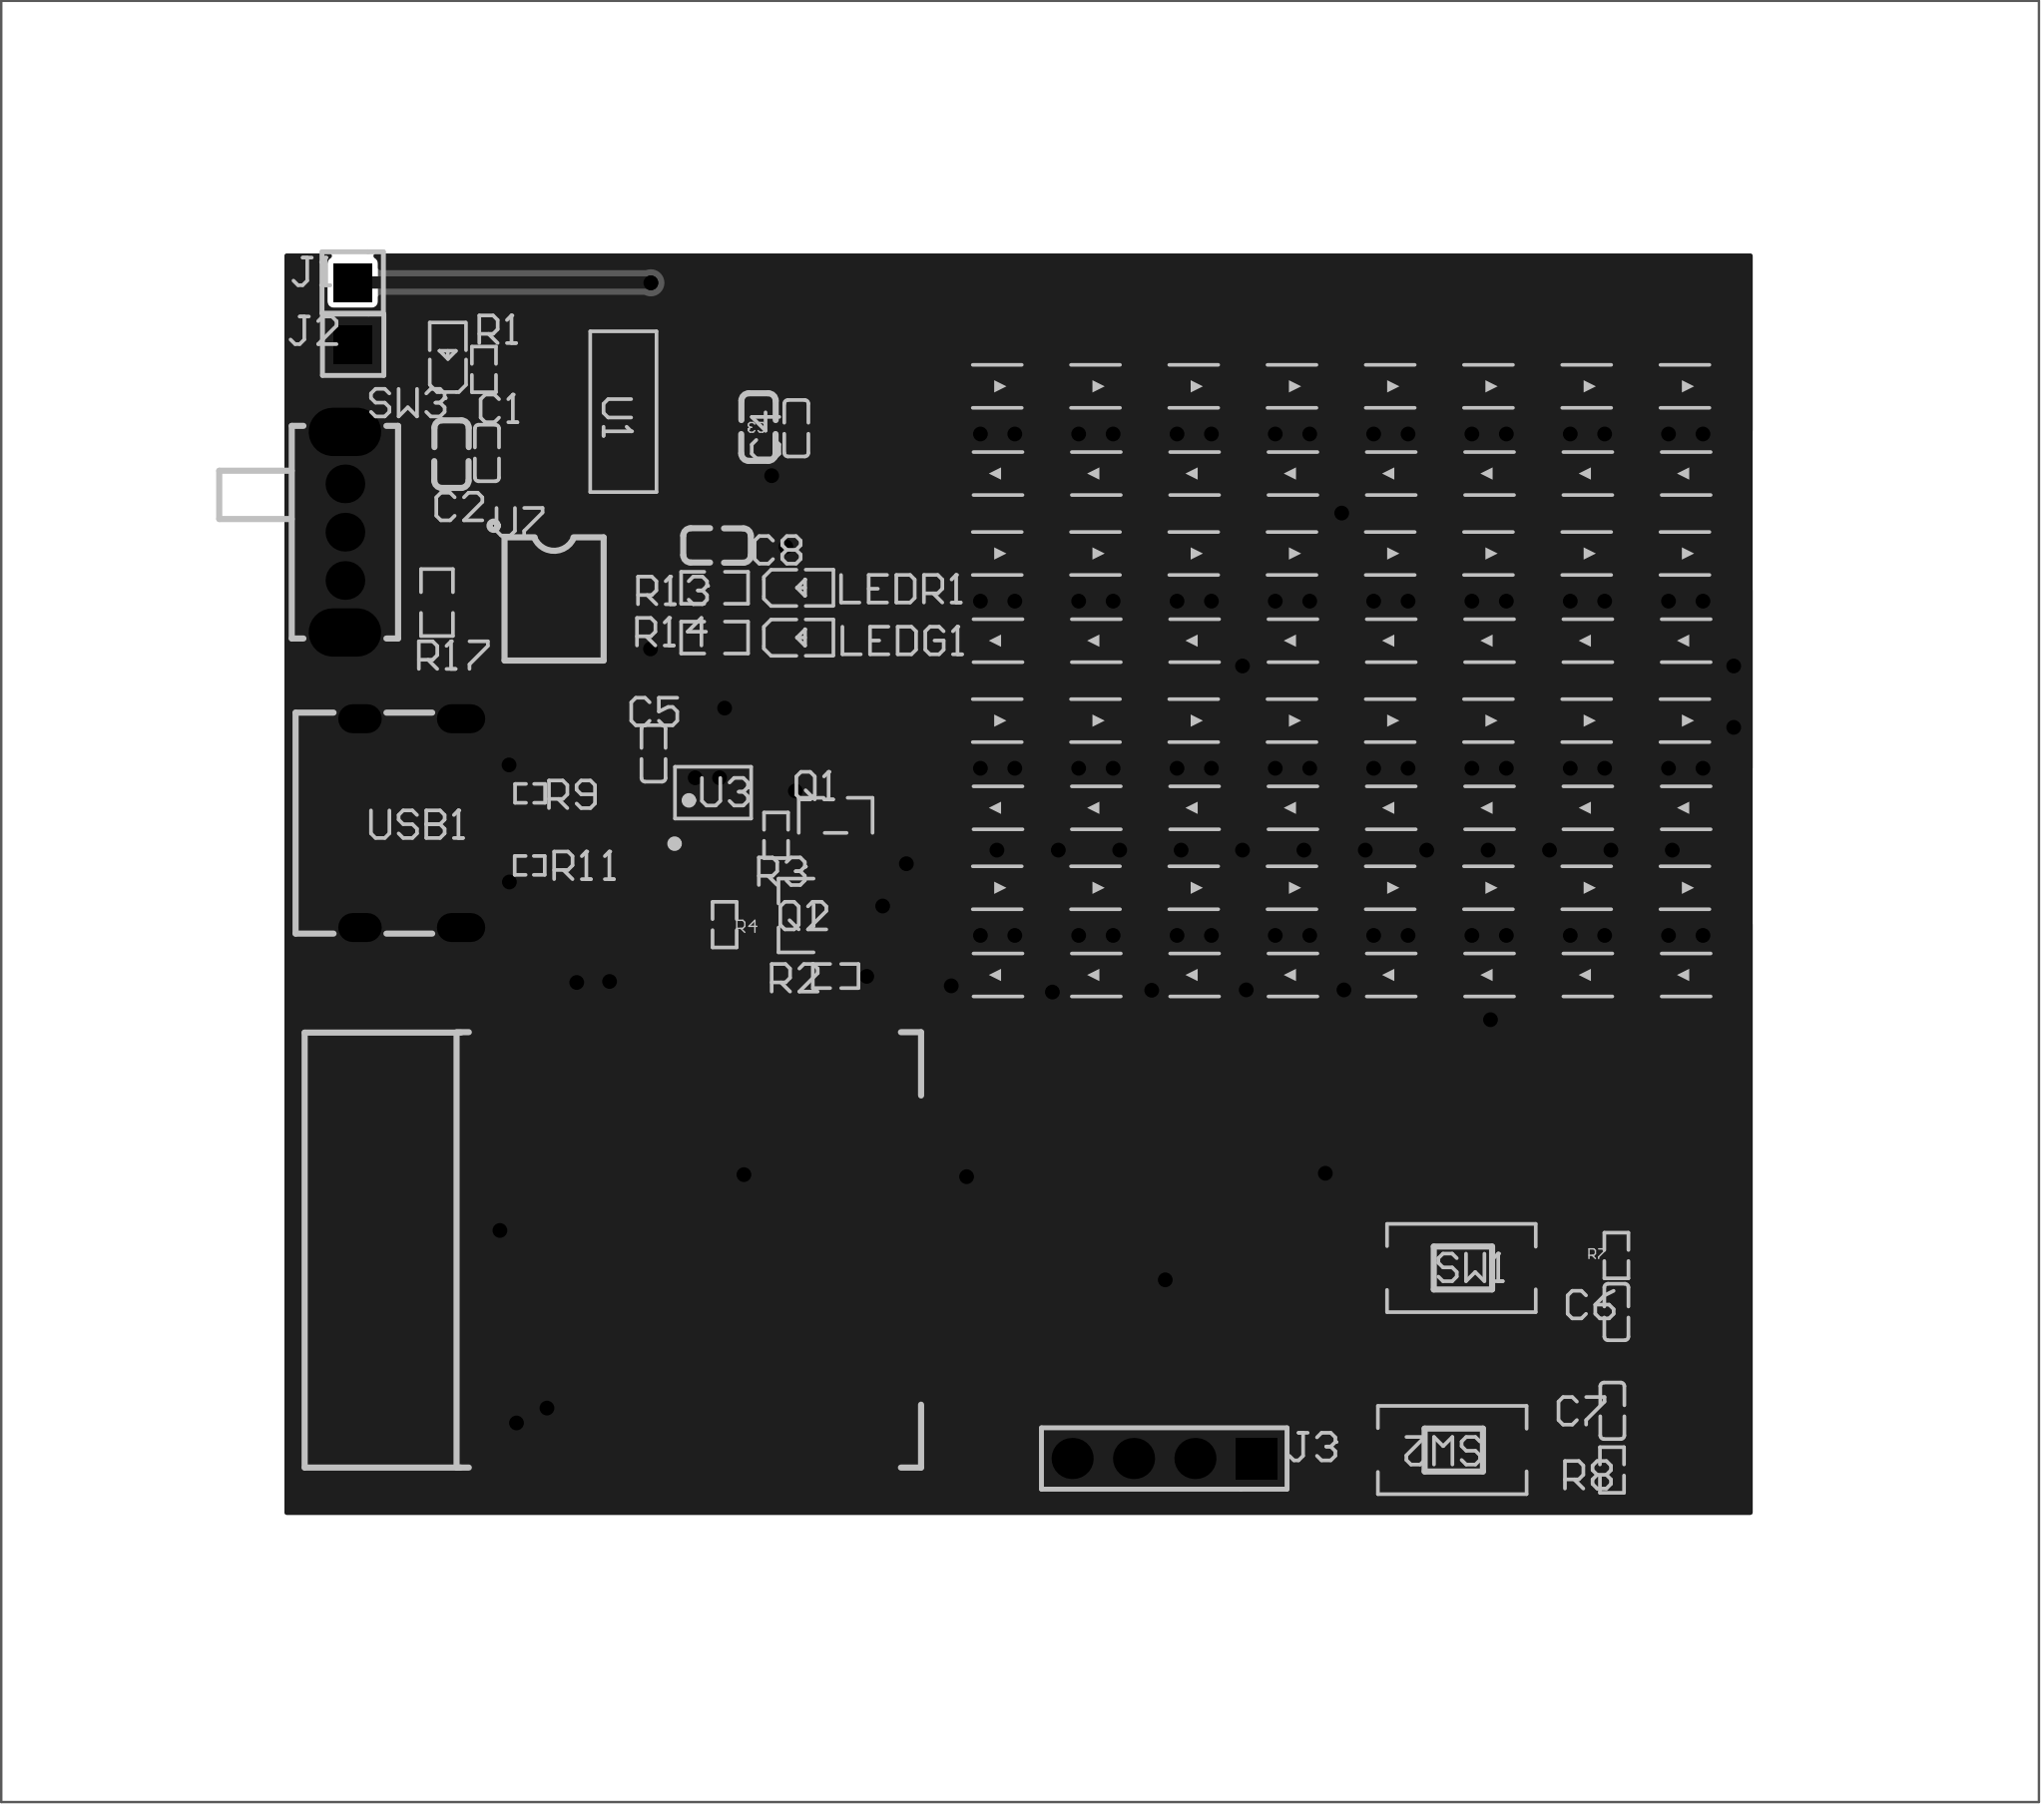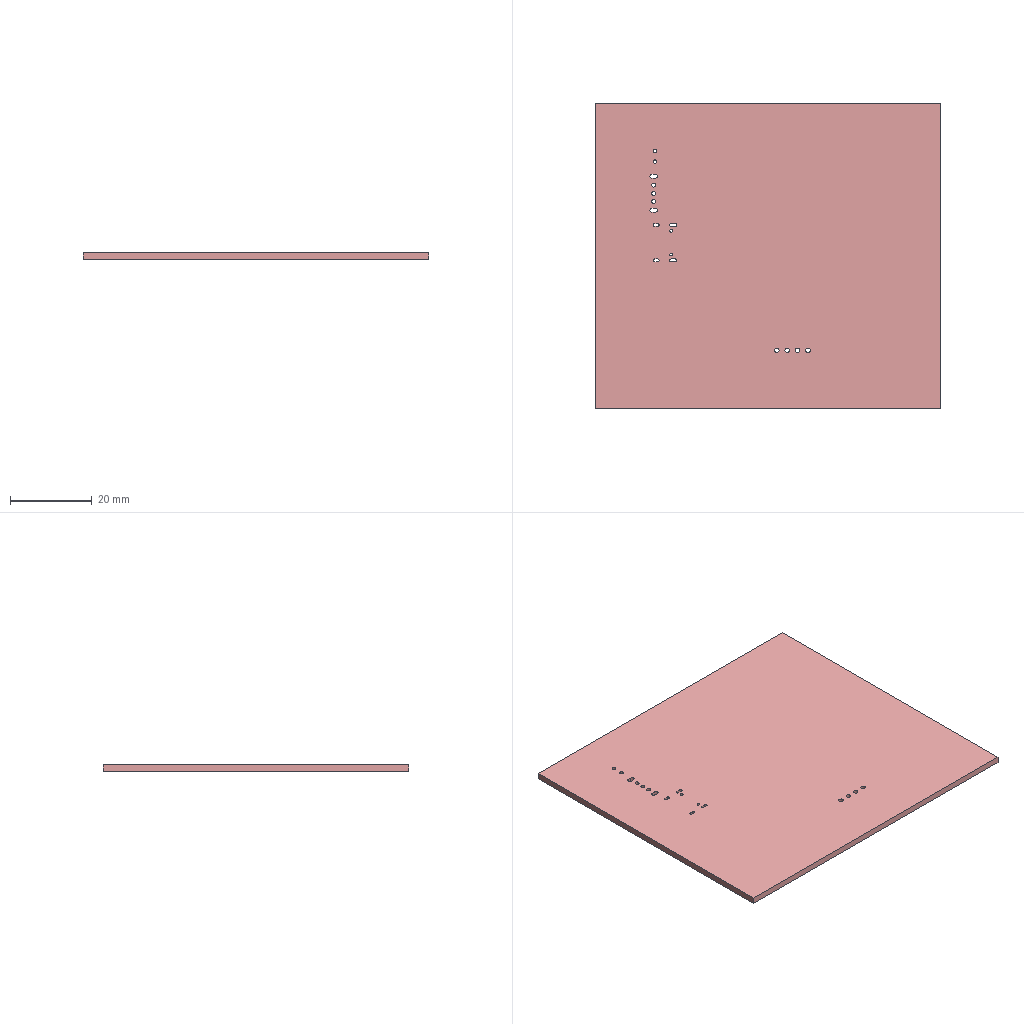Circuit board layout | Altium Designer | box 84.3 x 74.5 x 1.6 mm
Layer stack:
# Altium Designer layer stack of  (unit mm; dielectric type: 0 none, 1 core, 2 prepreg, 3 surface material)
index,name,kind,layer,copper_thickness_mm,dielectric_type,dielectric_thickness_mm,dielectric_material,dielectric_constant
0,Top Paste Mask Layer,other,,,,,,
1,Top Silkscreen Layer,other,,,,,,
2,Top Solder Mask Layer,dielectric,,,3,0.01,,3.3
3,Top Layer,copper,Top Layer,0.035,,,,
4,Dielectric1,dielectric,,,3,1.51,FR4,4.5
5,Bottom Layer,copper,Bottom Layer,0.035,,,,
6,Bottom Solder Mask Layer,dielectric,,,3,0.01,,3.3
7,Bottom Silkscreen Layer,other,,,,,,
8,Bottom Paste Mask Layer,other,,,,,,
# drill layer pairs: low layer,high layer
drill_pair,Top Layer,Bottom Layer
Part placement:
Designator,Comment,Layer,Footprint,Center-X(mm),Center-Y(mm),Rotation
C6,100nF,TopLayer,C0402,136.666,90.13,270
C1,100nF,TopLayer,C0402,89.944,125.677,90
C2,22uF,TopLayer,C0603,88.475,125.622,270
C7,100nF,TopLayer,C0402,136.498,86.042,90
C3,22uF,TopLayer,C0603,101.173,126.742,270
C5,100nF,TopLayer,C0402,96.834,113.243,90
C4,100nF,TopLayer,C0402,102.742,126.701,90
J3,2.54-1*4,TopLayer,HDR-TH_4P-P2.54-V-M-1,117.962,84.068,180
LED1,XL-1608SURC-06,TopLayer,LED0603-RD_RED,88.333,129.687,90
Q1,SS8050-G,TopLayer,SOT-23-3_L2.9-W1.3-P1.90-LS2.4-BR,104.368,110.682,270
Q2,SS8050-G,TopLayer,SOT-23-3_L2.9-W1.3-P1.90-LS2.4-BR,102.73,106.538,0
R1,2kΩ,TopLayer,R0402,89.819,129.136,270
R7,10kΩ,TopLayer,R0402,136.666,92.468,270
R3,10kΩ,TopLayer,R0402,101.904,109.856,90
R4,10kΩ,TopLayer,R0402,99.775,106.159,270
R8,10kΩ,TopLayer,R0402,136.484,83.592,90
R9,5.1kΩ,TopLayer,R0201,91.727,111.592,180
R11,5.1kΩ,TopLayer,R0201,91.713,108.61,0
R2,10kΩ,TopLayer,R0402,104.368,104.032,0
SW1,TSB008A2530A,TopLayer,SW-SMD_L6.0-W3.5-LS8.0,130.254,91.95,0
SW2,TSB008A2530A,TopLayer,SW-SMD_L6.0-W3.5-LS8.0,129.876,84.418,0
U3,CH340E,TopLayer,MSOP-10_L3.0-W3.0-P0.50-LS5.0-BL,99.297,111.62,0
U1,AMS1117-3.3,TopLayer,SOT-223-4_L6.5-W3.5-P2.30-LS7.0-BR,95.587,127.386,180
U2,ESP32-WROOM-32E-N16,TopLayer,WIFI-SMD_ESP32-WROOM-32E,98.879,92.692,0
USB1,KH-TYPE-C-16P-T,TopLayer,USB-C-SMD_KH-TYPE-C-16P,87.107,110.36,270
C8,100nF,TopLayer,C0603,99.454,121.854,180
J1,HDR-M-2.54_1x1,TopLayer,HDR-M-2.54_1X1,84.39,132.732,90
J2,HDR-M-2.54_1x1,TopLayer,HDR-M-2.54_1X1,84.409,130.155,90
LEDG1,,TopLayer,LED_0603,102.886,118.031,0
LEDR1,,TopLayer,LED_0603,102.886,120.092,0
R13,1K,TopLayer,R0603,99.361,120.099,0
R14,1K,TopLayer,R0603,99.361,118.038,0
R17,1.2K,TopLayer,R0603,87.876,119.488,90
U7,TP4056,TopLayer,ESOP-8_L4.9-W3.9-P1.27-LS6.0-BL-EP,92.721,119.637,270
SW3,,TopLayer,拨动开关_侧,84.068,122.4,270
LED2,WS2812B-0807幻彩,TopLayer,LED-SMD_4P-L2.0-W1.8-TL,135.486,104.076,0
LED2,WS2812B-0807幻彩,TopLayer,LED-SMD_4P-L2.0-W1.8-TL,139.553,104.076,0
LED2,WS2812B-0807幻彩,TopLayer,LED-SMD_4P-L2.0-W1.8-TL,127.352,104.076,0
LED2,WS2812B-0807幻彩,TopLayer,LED-SMD_4P-L2.0-W1.8-TL,131.419,104.076,0
LED2,WS2812B-0807幻彩,TopLayer,LED-SMD_4P-L2.0-W1.8-TL,119.219,104.076,0
LED2,WS2812B-0807幻彩,TopLayer,LED-SMD_4P-L2.0-W1.8-TL,123.285,104.076,0
LED2,WS2812B-0807幻彩,TopLayer,LED-SMD_4P-L2.0-W1.8-TL,115.152,104.076,0
LED2,WS2812B-0807幻彩,TopLayer,LED-SMD_4P-L2.0-W1.8-TL,127.31,107.685,180
LED2,WS2812B-0807幻彩,TopLayer,LED-SMD_4P-L2.0-W1.8-TL,135.438,107.685,180
LED2,WS2812B-0807幻彩,TopLayer,LED-SMD_4P-L2.0-W1.8-TL,123.246,107.685,180
LED2,WS2812B-0807幻彩,TopLayer,LED-SMD_4P-L2.0-W1.8-TL,139.502,107.685,180
LED2,WS2812B-0807幻彩,TopLayer,LED-SMD_4P-L2.0-W1.8-TL,131.374,107.685,180
LED2,WS2812B-0807幻彩,TopLayer,LED-SMD_4P-L2.0-W1.8-TL,115.118,107.685,180
LED2,WS2812B-0807幻彩,TopLayer,LED-SMD_4P-L2.0-W1.8-TL,119.182,107.685,180
LED2,WS2812B-0807幻彩,TopLayer,LED-SMD_4P-L2.0-W1.8-TL,123.285,110.993,0
LED2,WS2812B-0807幻彩,TopLayer,LED-SMD_4P-L2.0-W1.8-TL,115.152,110.993,0
LED2,WS2812B-0807幻彩,TopLayer,LED-SMD_4P-L2.0-W1.8-TL,139.553,110.993,0
LED2,WS2812B-0807幻彩,TopLayer,LED-SMD_4P-L2.0-W1.8-TL,135.486,110.993,0
LED2,WS2812B-0807幻彩,TopLayer,LED-SMD_4P-L2.0-W1.8-TL,127.352,110.993,0
LED2,WS2812B-0807幻彩,TopLayer,LED-SMD_4P-L2.0-W1.8-TL,131.419,110.993,0
LED2,WS2812B-0807幻彩,TopLayer,LED-SMD_4P-L2.0-W1.8-TL,119.219,110.993,0
LED2,WS2812B-0807幻彩,TopLayer,LED-SMD_4P-L2.0-W1.8-TL,135.438,121.518,180
LED2,WS2812B-0807幻彩,TopLayer,LED-SMD_4P-L2.0-W1.8-TL,127.31,121.518,180
LED2,WS2812B-0807幻彩,TopLayer,LED-SMD_4P-L2.0-W1.8-TL,131.374,121.518,180
LED2,WS2812B-0807幻彩,TopLayer,LED-SMD_4P-L2.0-W1.8-TL,119.182,121.518,180
LED2,WS2812B-0807幻彩,TopLayer,LED-SMD_4P-L2.0-W1.8-TL,115.118,121.518,180
LED2,WS2812B-0807幻彩,TopLayer,LED-SMD_4P-L2.0-W1.8-TL,139.502,121.518,180
LED2,WS2812B-0807幻彩,TopLayer,LED-SMD_4P-L2.0-W1.8-TL,123.246,121.518,180
LED2,WS2812B-0807幻彩,TopLayer,LED-SMD_4P-L2.0-W1.8-TL,139.553,117.91,0
LED2,WS2812B-0807幻彩,TopLayer,LED-SMD_4P-L2.0-W1.8-TL,135.486,117.91,0
LED2,WS2812B-0807幻彩,TopLayer,LED-SMD_4P-L2.0-W1.8-TL,115.118,128.435,180
LED2,WS2812B-0807幻彩,TopLayer,LED-SMD_4P-L2.0-W1.8-TL,135.438,128.435,180
LED2,WS2812B-0807幻彩,TopLayer,LED-SMD_4P-L2.0-W1.8-TL,127.31,128.435,180
LED2,WS2812B-0807幻彩,TopLayer,LED-SMD_4P-L2.0-W1.8-TL,131.374,128.435,180
LED2,WS2812B-0807幻彩,TopLayer,LED-SMD_4P-L2.0-W1.8-TL,119.182,128.435,180
LED2,WS2812B-0807幻彩,TopLayer,LED-SMD_4P-L2.0-W1.8-TL,123.246,128.435,180
LED2,WS2812B-0807幻彩,TopLayer,LED-SMD_4P-L2.0-W1.8-TL,139.553,124.826,0
LED2,WS2812B-0807幻彩,TopLayer,LED-SMD_4P-L2.0-W1.8-TL,115.152,124.826,0
LED2,WS2812B-0807幻彩,TopLayer,LED-SMD_4P-L2.0-W1.8-TL,135.486,124.826,0
LED2,WS2812B-0807幻彩,TopLayer,LED-SMD_4P-L2.0-W1.8-TL,123.285,124.826,0
LED2,WS2812B-0807幻彩,TopLayer,LED-SMD_4P-L2.0-W1.8-TL,119.219,124.826,0
LED2,WS2812B-0807幻彩,TopLayer,LED-SMD_4P-L2.0-W1.8-TL,131.419,124.826,0
LED2,WS2812B-0807幻彩,TopLayer,LED-SMD_4P-L2.0-W1.8-TL,127.352,124.826,0
LED2,WS2812B-0807幻彩,TopLayer,LED-SMD_4P-L2.0-W1.8-TL,123.285,117.91,0
LED2,WS2812B-0807幻彩,TopLayer,LED-SMD_4P-L2.0-W1.8-TL,115.152,117.91,0
LED2,WS2812B-0807幻彩,TopLayer,LED-SMD_4P-L2.0-W1.8-TL,127.352,117.91,0
LED2,WS2812B-0807幻彩,TopLayer,LED-SMD_4P-L2.0-W1.8-TL,119.219,117.91,0
LED2,WS2812B-0807幻彩,TopLayer,LED-SMD_4P-L2.0-W1.8-TL,139.502,114.601,180
LED2,WS2812B-0807幻彩,TopLayer,LED-SMD_4P-L2.0-W1.8-TL,127.31,114.601,180
LED2,WS2812B-0807幻彩,TopLayer,LED-SMD_4P-L2.0-W1.8-TL,135.438,114.601,180
LED2,WS2812B-0807幻彩,TopLayer,LED-SMD_4P-L2.0-W1.8-TL,123.246,114.601,180
LED2,WS2812B-0807幻彩,TopLayer,LED-SMD_4P-L2.0-W1.8-TL,131.374,114.601,180
LED2,WS2812B-0807幻彩,TopLayer,LED-SMD_4P-L2.0-W1.8-TL,115.118,114.601,180
LED2,WS2812B-0807幻彩,TopLayer,LED-SMD_4P-L2.0-W1.8-TL,119.182,114.601,180
LED2,WS2812B-0807幻彩,TopLayer,LED-SMD_4P-L2.0-W1.8-TL,139.502,128.435,180
LED2,WS2812B-0807幻彩,TopLayer,LED-SMD_4P-L2.0-W1.8-TL,131.419,117.91,0
LED2,WS2812B-0807幻彩,TopLayer,LED-SMD_4P-L2.0-W1.8-TL,111.085,117.91,0
LED2,WS2812B-0807幻彩,TopLayer,LED-SMD_4P-L2.0-W1.8-TL,111.085,110.993,0
LED2,WS2812B-0807幻彩,TopLayer,LED-SMD_4P-L2.0-W1.8-TL,111.085,124.826,0
LED2,WS2812B-0807幻彩,TopLayer,LED-SMD_4P-L2.0-W1.8-TL,111.085,104.076,0
LED2,WS2812B-0807幻彩,TopLayer,LED-SMD_4P-L2.0-W1.8-TL,111.054,128.435,180
LED2,WS2812B-0807幻彩,TopLayer,LED-SMD_4P-L2.0-W1.8-TL,111.054,107.685,180
LED2,WS2812B-0807幻彩,TopLayer,LED-SMD_4P-L2.0-W1.8-TL,111.054,121.518,180
LED2,WS2812B-0807幻彩,TopLayer,LED-SMD_4P-L2.0-W1.8-TL,111.054,114.601,180
Pad and via stacks:
# Altium Designer via and pad stacks of  (unit mm). Each distinct definition once, with the count of objects using it.
# via: kind,start_layer,end_layer,hole_mm,diameter_mm,mode(0 simple;1 top-mid-bottom;2 full stack),diameter_per_layer,count,example_net
# pad: kind,layer,hole_mm,hole_type(0 round;1 square;2 slot),plating,top_size,top_shape(1 round;2 rect;3 octagon;9 rounded rect),mid_size,bottom_size,mode,footprint,size_per_layer,count,example
pad,Top Layer,0,0,plated,0.7901x0.54,2,0.7901x0.54,0.7901x0.54,0,C0402,,10,C6.2
pad,Top Layer,0,0,plated,0.8x0.9,2,0.8x0.9,0.8x0.9,0,C0603,,6,C2.2
pad,Top Layer,0,0,plated,0.8x0.8,2,0.8x0.8,0.8x0.8,0,LED0603-RD_RED,,2,LED1.1
pad,Top Layer,0,0,plated,1.25x0.7,2,1.25x0.7,1.25x0.7,0,SOT-23-3_L2.9-W1.3-P1.90-LS2.4-BR,,6,Q1.1
pad,Top Layer,0,0,plated,0.5657x0.54,2,0.5657x0.54,0.5657x0.54,0,R0402,,12,R1.2
pad,Top Layer,0,0,plated,0.3031x0.324,2,0.3031x0.324,0.3031x0.324,0,R0201,,4,R9.2
pad,Top Layer,0,0,plated,1.74x1.4,2,1.74x1.4,1.74x1.4,0,SW-SMD_L6.0-W3.5-LS8.0,,4,SW1.1
pad,Top Layer,0,0,plated,0.28x1.62,1,0.28x1.62,0.28x1.62,0,MSOP-10_L3.0-W3.0-P0.50-LS5.0-BL,,10,U3.1
pad,Top Layer,0,0,plated,2.47x0.98,2,2.47x0.98,2.47x0.98,0,SOT-223-4_L6.5-W3.5-P2.30-LS7.0-BR,,3,U1.1
pad,Top Layer,0,0,plated,2.47x3.6,2,2.47x3.6,2.47x3.6,0,SOT-223-4_L6.5-W3.5-P2.30-LS7.0-BR,,1,U1.4
pad,Top Layer,0,0,plated,0.95x2.1,2,0.95x2.1,0.95x2.1,0,WIFI-SMD_ESP32-WROOM-32E,,28,U2.1
pad,Top Layer,0,0,plated,2.1x0.95,2,2.1x0.95,2.1x0.95,0,WIFI-SMD_ESP32-WROOM-32E,,10,U2.15
pad,Top Layer,0,0,plated,0.9x0.9,2,0.9x0.9,0.9x0.9,0,WIFI-SMD_ESP32-WROOM-32E,,9,U2.39
pad,Top Layer,0,0,plated,0.3x1.3,2,0.3x1.3,0.3x1.3,0,USB-C-SMD_KH-TYPE-C-16P,,16,USB1.A1
pad,Top Layer,0,0,plated,0.8001x0.8001,2,0.8001x0.8001,0.8001x0.8001,0,LED_0603,,4,LEDG1.1
pad,Top Layer,0,0,plated,0.8065x0.864,2,0.8065x0.864,0.8065x0.864,0,R0603,,6,R13.2
pad,Top Layer,0,0,plated,0.6x1.2,2,0.6x1.2,0.6x1.2,0,ESOP-8_L4.9-W3.9-P1.27-LS6.0-BL-EP,,8,U7.1
pad,Top Layer,0,0,plated,3.3x2.4,2,3.3x2.4,3.3x2.4,0,ESOP-8_L4.9-W3.9-P1.27-LS6.0-BL-EP,,1,U7.9
pad,Top Layer,0,0,plated,1x0.5,2,1x0.5,1x0.5,0,LED-SMD_4P-L2.0-W1.8-TL,,256,LED2.1
pad,Multi-Layer,1.1,0,plated,1.7x1.7,2,1.7x1.7,1.7x1.7,0,HDR-TH_4P-P2.54-V-M-1,,1,J3.1
pad,Multi-Layer,1.1,0,plated,1.7x1.7,1,1.7x1.7,1.7x1.7,0,HDR-TH_4P-P2.54-V-M-1,,3,J3.2
pad,Multi-Layer,0.7,2,plated,1.2x1.8,1,1.2x1.8,1.2x1.8,0,USB-C-SMD_KH-TYPE-C-16P,,2,USB1.3
pad,Multi-Layer,0.7,2,plated,1.2x2,1,1.2x2,1.2x2,0,USB-C-SMD_KH-TYPE-C-16P,,2,USB1.2
pad,Multi-Layer,0.889,0,plated,1.575x1.575,2,1.575x1.575,1.575x1.575,0,HDR-M-2.54_1X1,,2,J1.1
pad,Multi-Layer,1.001,0,plated,1.6x1.6,1,1.6x1.6,1.6x1.6,0,\u00B2\u00A6\u00B6\u00AF\u00BF\u00AA\u00B9\u00D8_\u00B2\u00E0,,3,SW3.1
pad,Multi-Layer,1.001,2,plated,3x1.999,1,3x1.999,3x1.999,0,\u00B2\u00A6\u00B6\u00AF\u00BF\u00AA\u00B9\u00D8_\u00B2\u00E0,,2,SW3.4
pad,Bottom Layer,0,0,plated,0.8x0.9,2,0.8x0.9,0.8x0.9,0,LED-SMD_4P-L2.0-W1.8-TL,,128,LED2.5
via,Top Layer,Bottom Layer,0.3048,0.61,0,,112,GND
Copper pours:
name,layer,net,type(0 solid;1 hatched;2 none)
Top Layer-GND,Top Layer,GND,0
Bottom Layer-GND,Bottom Layer,GND,0
Design rules, without the lines most boards share:
# Altium Designer design rules of  (exported by Altium Designer, unit mm)
# columns: name | kind | enabled | priority | scope1 | scope2 | descriptor | typed fields (field=value)
Plane_Default | 0 | disabled | 1 | All | All | Clearance Constraint (Gap=5.984mil) (Disabled)(All),(All) | gap=0.152
Plane_Default_1 | 63 | disabled | 1 | All | All | Board Clearance Constraint (Gap=0mil) (Disabled)(All) |
Copper_gge30915 | 0 | disabled | 2 | All | All | Clearance Constraint (Gap=5.984mil) (Disabled)(All),(All) | gap=0.152
Copper_gge30915_1 | 63 | disabled | 2 | All | All | Board Clearance Constraint (Gap=0mil) (Disabled)(All) |
Copper_gge30960 | 0 | disabled | 3 | All | All | Clearance Constraint (Gap=5.984mil) (Disabled)(All),(All) | gap=0.152
Copper_gge30960_1 | 63 | disabled | 3 | All | All | Board Clearance Constraint (Gap=0mil) (Disabled)(All) |
Default | 0 | enabled | 4 | All | All | Clearance Constraint (Gap=5.984mil) (All),(All) | gap=0.152
Default_1 | 63 | enabled | 4 | All | All | Board Clearance Constraint (Gap=0mil) (All) |
otherClearance | 52 | enabled | 1 | All | All | Hole To Hole Clearance (Gap=11.8mil) (All),(All) | gap=0.2997
Default_2 | 2 | enabled | 1 | All | All | Width Constraint (Min=10mil) (Max=1000mil) (Preferred=10mil) (All) |
Default_3 | 11 | enabled | 1 | All | All | Routing Via (MinHoleWidth=12.008mil) (MaxHoleWidth=2362mil) (PreferredHoleWidth=12.008mil) (MinWidth=24.016mil) (MaxWidth=3938mil) (PreferedWidth=24.016mil) (All) | via_min_hole=0.305 via_max_hole=59.995 via_preferred_diameter=0.61 via_preferred_hole=0.305
Default_4 | 6 | enabled | 1 | All | All | Power Plane Connect Rule(Relief Connect )(Expansion=20mil) (Conductor Width=0mil) (Air Gap=10mil) (Entries=4) (All) | relief_conductor_width=0 relief_entries=4 relief_expansion=0.508
gge30960 | 20 | disabled | 1 | All | All | Polygon Connect Rule(Relief Connect )(Conductor Width=0mil) (Relief Angle=90 Angle) (Entries=4) (Air Gap Width=10mil) (Disabled)(All),(All) | connect_style(0=relief,1=direct,2=none)=0 relief_conductor_width=0 relief_entries=4
gge30915 | 20 | enabled | 2 | All | All | Polygon Connect Rule(Relief Connect )(Conductor Width=0mil) (Relief Angle=90 Angle) (Entries=4) (Air Gap Width=10mil) (All),(All) | connect_style(0=relief,1=direct,2=none)=0 relief_conductor_width=0 relief_entries=4
Common | 14 | enabled | 1 | All | All | Paste Mask Expansion (Expansion =0mil) (All) | expansion=0
Common_1 | 13 | enabled | 2 | All | All | Solder Mask Expansion (Expansion =2mil) (All) | expansion=0.0508
Common_2 | 13 | enabled | 1 | IsVia | All | Solder Mask Expansion (Expansion =-1000mil) (IsVia) | expansion=-25.4